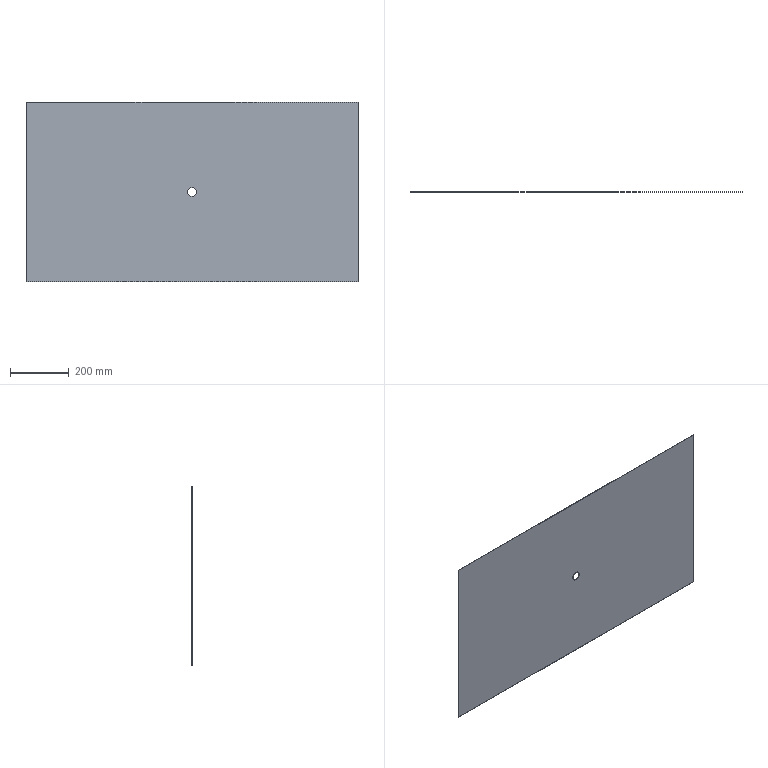Part | SolidWorks | features EdgeFlange 2, FlatPattern 1, ICE 1, SMBaseFlange 1, SheetMetal 1 | 1 solid | 8 faces | box 1135 x 1.2 x 615 mm | volume 836782 mm3 | plane 6 | cylinder 2 | commonest cylinder face diameters 30 x2
STEP:
#1=CARTESIAN_POINT('',(0.,-1.2,-15.));
#2=VERTEX_POINT('',#1);
#3=CARTESIAN_POINT('',(0.,-1.2,15.));
#4=VERTEX_POINT('',#3);
#5=CARTESIAN_POINT('',(0.,-1.2,0.));
#6=DIRECTION('',(0.,1.,0.));
#7=DIRECTION('',(0.,0.,1.));
#8=AXIS2_PLACEMENT_3D('',#5,#6,#7);
#9=CIRCLE('',#8,15.);
#10=EDGE_CURVE('',#2,#4,#9,.T.);
#11=ORIENTED_EDGE('',*,*,#10,.F.);
#12=CARTESIAN_POINT('',(0.,0.,-15.));
#13=VERTEX_POINT('',#12);
#14=CARTESIAN_POINT('',(0.,-10.,-15.));
#15=DIRECTION('',(0.,1.,0.));
#16=VECTOR('',#15,1000.);
#17=LINE('',#14,#16);
#18=EDGE_CURVE('',#2,#13,#17,.T.);
#19=ORIENTED_EDGE('',*,*,#18,.T.);
#20=CARTESIAN_POINT('',(0.,0.,15.));
#21=VERTEX_POINT('',#20);
#22=CARTESIAN_POINT('',(0.,0.,0.));
#23=DIRECTION('',(0.,1.,0.));
#24=DIRECTION('',(0.,0.,1.));
#25=AXIS2_PLACEMENT_3D('',#22,#23,#24);
#26=CIRCLE('',#25,15.);
#27=EDGE_CURVE('',#13,#21,#26,.T.);
#28=ORIENTED_EDGE('',*,*,#27,.T.);
#29=CARTESIAN_POINT('',(0.,-10.,15.));
#30=DIRECTION('',(0.,1.,0.));
#31=VECTOR('',#30,1000.);
#32=LINE('',#29,#31);
#33=EDGE_CURVE('',#4,#21,#32,.T.);
#34=ORIENTED_EDGE('',*,*,#33,.F.);
#35=EDGE_LOOP('',(#11,#19,#28,#34));
#36=FACE_OUTER_BOUND('',#35,.T.);
#37=CARTESIAN_POINT('',(0.,-10.,0.));
#38=DIRECTION('',(0.,1.,0.));
#39=DIRECTION('',(0.,0.,1.));
#40=AXIS2_PLACEMENT_3D('',#37,#38,#39);
#41=CYLINDRICAL_SURFACE('',#40,15.);
#42=ADVANCED_FACE('',(#36),#41,.F.);
#43=CARTESIAN_POINT('',(567.5,0.,307.5));
#44=VERTEX_POINT('',#43);
#45=CARTESIAN_POINT('',(567.5,0.,-307.5));
#46=VERTEX_POINT('',#45);
#47=CARTESIAN_POINT('',(567.5,0.,-307.5));
#48=DIRECTION('',(0.,0.,-1.));
#49=VECTOR('',#48,1000.);
#50=LINE('',#47,#49);
#51=EDGE_CURVE('',#44,#46,#50,.T.);
#52=ORIENTED_EDGE('',*,*,#51,.F.);
#53=CARTESIAN_POINT('',(567.5,-1.2,307.5));
#54=VERTEX_POINT('',#53);
#55=CARTESIAN_POINT('',(567.5,-1.2,307.5));
#56=DIRECTION('',(0.,1.,0.));
#57=VECTOR('',#56,1000.);
#58=LINE('',#55,#57);
#59=EDGE_CURVE('',#54,#44,#58,.T.);
#60=ORIENTED_EDGE('',*,*,#59,.F.);
#61=CARTESIAN_POINT('',(567.5,-1.2,-307.5));
#62=VERTEX_POINT('',#61);
#63=CARTESIAN_POINT('',(567.5,-1.2,-307.5));
#64=DIRECTION('',(0.,0.,-1.));
#65=VECTOR('',#64,1000.);
#66=LINE('',#63,#65);
#67=EDGE_CURVE('',#54,#62,#66,.T.);
#68=ORIENTED_EDGE('',*,*,#67,.T.);
#69=CARTESIAN_POINT('',(567.5,-1.2,-307.5));
#70=DIRECTION('',(0.,1.,0.));
#71=VECTOR('',#70,1000.);
#72=LINE('',#69,#71);
#73=EDGE_CURVE('',#62,#46,#72,.T.);
#74=ORIENTED_EDGE('',*,*,#73,.T.);
#75=EDGE_LOOP('',(#52,#60,#68,#74));
#76=FACE_OUTER_BOUND('',#75,.T.);
#77=CARTESIAN_POINT('',(567.5,-1.2,-307.5));
#78=DIRECTION('',(1.,0.,0.));
#79=DIRECTION('',(0.,0.,-1.));
#80=AXIS2_PLACEMENT_3D('',#77,#78,#79);
#81=PLANE('',#80);
#82=ADVANCED_FACE('',(#76),#81,.T.);
#83=CARTESIAN_POINT('',(-567.5,0.,307.5));
#84=VERTEX_POINT('',#83);
#85=CARTESIAN_POINT('',(-567.5,0.,307.5));
#86=DIRECTION('',(1.,0.,0.));
#87=VECTOR('',#86,1000.);
#88=LINE('',#85,#87);
#89=EDGE_CURVE('',#84,#44,#88,.T.);
#90=ORIENTED_EDGE('',*,*,#89,.F.);
#91=CARTESIAN_POINT('',(-567.5,-1.2,307.5));
#92=VERTEX_POINT('',#91);
#93=CARTESIAN_POINT('',(-567.5,-1.2,307.5));
#94=DIRECTION('',(0.,1.,0.));
#95=VECTOR('',#94,1000.);
#96=LINE('',#93,#95);
#97=EDGE_CURVE('',#92,#84,#96,.T.);
#98=ORIENTED_EDGE('',*,*,#97,.F.);
#99=CARTESIAN_POINT('',(-567.5,-1.2,307.5));
#100=DIRECTION('',(1.,0.,0.));
#101=VECTOR('',#100,1000.);
#102=LINE('',#99,#101);
#103=EDGE_CURVE('',#92,#54,#102,.T.);
#104=ORIENTED_EDGE('',*,*,#103,.T.);
#105=ORIENTED_EDGE('',*,*,#59,.T.);
#106=EDGE_LOOP('',(#90,#98,#104,#105));
#107=FACE_OUTER_BOUND('',#106,.T.);
#108=CARTESIAN_POINT('',(-567.5,-1.2,307.5));
#109=DIRECTION('',(0.,0.,1.));
#110=DIRECTION('',(1.,0.,0.));
#111=AXIS2_PLACEMENT_3D('',#108,#109,#110);
#112=PLANE('',#111);
#113=ADVANCED_FACE('',(#107),#112,.T.);
#114=CARTESIAN_POINT('',(-567.5,0.,-307.5));
#115=VERTEX_POINT('',#114);
#116=CARTESIAN_POINT('',(-567.5,0.,-307.5));
#117=DIRECTION('',(0.,0.,1.));
#118=VECTOR('',#117,1000.);
#119=LINE('',#116,#118);
#120=EDGE_CURVE('',#115,#84,#119,.T.);
#121=ORIENTED_EDGE('',*,*,#120,.F.);
#122=CARTESIAN_POINT('',(-567.5,-1.2,-307.5));
#123=VERTEX_POINT('',#122);
#124=CARTESIAN_POINT('',(-567.5,-1.2,-307.5));
#125=DIRECTION('',(0.,1.,0.));
#126=VECTOR('',#125,1000.);
#127=LINE('',#124,#126);
#128=EDGE_CURVE('',#123,#115,#127,.T.);
#129=ORIENTED_EDGE('',*,*,#128,.F.);
#130=CARTESIAN_POINT('',(-567.5,-1.2,-307.5));
#131=DIRECTION('',(0.,0.,1.));
#132=VECTOR('',#131,1000.);
#133=LINE('',#130,#132);
#134=EDGE_CURVE('',#123,#92,#133,.T.);
#135=ORIENTED_EDGE('',*,*,#134,.T.);
#136=ORIENTED_EDGE('',*,*,#97,.T.);
#137=EDGE_LOOP('',(#121,#129,#135,#136));
#138=FACE_OUTER_BOUND('',#137,.T.);
#139=CARTESIAN_POINT('',(-567.5,-1.2,-307.5));
#140=DIRECTION('',(-1.,0.,0.));
#141=DIRECTION('',(0.,0.,1.));
#142=AXIS2_PLACEMENT_3D('',#139,#140,#141);
#143=PLANE('',#142);
#144=ADVANCED_FACE('',(#138),#143,.T.);
#145=CARTESIAN_POINT('',(-567.5,0.,-307.5));
#146=DIRECTION('',(-1.,0.,0.));
#147=VECTOR('',#146,1000.);
#148=LINE('',#145,#147);
#149=EDGE_CURVE('',#46,#115,#148,.T.);
#150=ORIENTED_EDGE('',*,*,#149,.F.);
#151=ORIENTED_EDGE('',*,*,#73,.F.);
#152=CARTESIAN_POINT('',(-567.5,-1.2,-307.5));
#153=DIRECTION('',(-1.,0.,0.));
#154=VECTOR('',#153,1000.);
#155=LINE('',#152,#154);
#156=EDGE_CURVE('',#62,#123,#155,.T.);
#157=ORIENTED_EDGE('',*,*,#156,.T.);
#158=ORIENTED_EDGE('',*,*,#128,.T.);
#159=EDGE_LOOP('',(#150,#151,#157,#158));
#160=FACE_OUTER_BOUND('',#159,.T.);
#161=CARTESIAN_POINT('',(-567.5,-1.2,-307.5));
#162=DIRECTION('',(0.,0.,-1.));
#163=DIRECTION('',(-1.,0.,0.));
#164=AXIS2_PLACEMENT_3D('',#161,#162,#163);
#165=PLANE('',#164);
#166=ADVANCED_FACE('',(#160),#165,.T.);
#167=CARTESIAN_POINT('',(0.,-1.2,0.));
#168=DIRECTION('',(0.,1.,0.));
#169=DIRECTION('',(0.,0.,1.));
#170=AXIS2_PLACEMENT_3D('',#167,#168,#169);
#171=CIRCLE('',#170,15.);
#172=EDGE_CURVE('',#4,#2,#171,.T.);
#173=ORIENTED_EDGE('',*,*,#172,.T.);
#174=ORIENTED_EDGE('',*,*,#10,.T.);
#175=EDGE_LOOP('',(#173,#174));
#176=FACE_BOUND('',#175,.T.);
#177=ORIENTED_EDGE('',*,*,#67,.F.);
#178=ORIENTED_EDGE('',*,*,#103,.F.);
#179=ORIENTED_EDGE('',*,*,#134,.F.);
#180=ORIENTED_EDGE('',*,*,#156,.F.);
#181=EDGE_LOOP('',(#177,#178,#179,#180));
#182=FACE_OUTER_BOUND('',#181,.T.);
#183=CARTESIAN_POINT('',(0.,-1.2,0.));
#184=DIRECTION('',(0.,1.,0.));
#185=DIRECTION('',(0.,0.,1.));
#186=AXIS2_PLACEMENT_3D('',#183,#184,#185);
#187=PLANE('',#186);
#188=ADVANCED_FACE('',(#176,#182),#187,.F.);
#189=CARTESIAN_POINT('',(0.,0.,0.));
#190=DIRECTION('',(0.,1.,0.));
#191=DIRECTION('',(0.,0.,1.));
#192=AXIS2_PLACEMENT_3D('',#189,#190,#191);
#193=CIRCLE('',#192,15.);
#194=EDGE_CURVE('',#21,#13,#193,.T.);
#195=ORIENTED_EDGE('',*,*,#194,.F.);
#196=ORIENTED_EDGE('',*,*,#27,.F.);
#197=EDGE_LOOP('',(#195,#196));
#198=FACE_BOUND('',#197,.T.);
#199=ORIENTED_EDGE('',*,*,#51,.T.);
#200=ORIENTED_EDGE('',*,*,#149,.T.);
#201=ORIENTED_EDGE('',*,*,#120,.T.);
#202=ORIENTED_EDGE('',*,*,#89,.T.);
#203=EDGE_LOOP('',(#199,#200,#201,#202));
#204=FACE_OUTER_BOUND('',#203,.T.);
#205=CARTESIAN_POINT('',(0.,0.,0.));
#206=DIRECTION('',(0.,1.,0.));
#207=DIRECTION('',(0.,0.,1.));
#208=AXIS2_PLACEMENT_3D('',#205,#206,#207);
#209=PLANE('',#208);
#210=ADVANCED_FACE('',(#198,#204),#209,.T.);
#211=ORIENTED_EDGE('',*,*,#18,.F.);
#212=ORIENTED_EDGE('',*,*,#172,.F.);
#213=ORIENTED_EDGE('',*,*,#33,.T.);
#214=ORIENTED_EDGE('',*,*,#194,.T.);
#215=EDGE_LOOP('',(#211,#212,#213,#214));
#216=FACE_OUTER_BOUND('',#215,.T.);
#217=CARTESIAN_POINT('',(0.,-10.,0.));
#218=DIRECTION('',(0.,1.,0.));
#219=DIRECTION('',(0.,0.,1.));
#220=AXIS2_PLACEMENT_3D('',#217,#218,#219);
#221=CYLINDRICAL_SURFACE('',#220,15.);
#222=ADVANCED_FACE('',(#216),#221,.F.);
#223=CLOSED_SHELL('',(#42,#82,#113,#144,#166,#188,#210,#222));
#224=MANIFOLD_SOLID_BREP('',#223);
#225=CARTESIAN_POINT('',(0.,0.,0.));
#226=DIRECTION('',(0.,0.,1.));
#227=DIRECTION('',(1.,0.,0.));
#228=AXIS2_PLACEMENT_3D('',#225,#226,#227);
#229=(LENGTH_UNIT()NAMED_UNIT(*)SI_UNIT(.MILLI.,.METRE.));
#230=UNCERTAINTY_MEASURE_WITH_UNIT(LENGTH_MEASURE(0.00001),#229,'','');
#231=(NAMED_UNIT(*)PLANE_ANGLE_UNIT()SI_UNIT($,.RADIAN.));
#232=(NAMED_UNIT(*)SI_UNIT($,.STERADIAN.)SOLID_ANGLE_UNIT());
#233=(GEOMETRIC_REPRESENTATION_CONTEXT(3)GLOBAL_UNCERTAINTY_ASSIGNED_CONTEXT((#230))GLOBAL_UNIT_ASSIGNED_CONTEXT((#229,#231,#232))REPRESENTATION_CONTEXT('',''));
#234=ADVANCED_BREP_SHAPE_REPRESENTATION('',(#224,#228),#233);